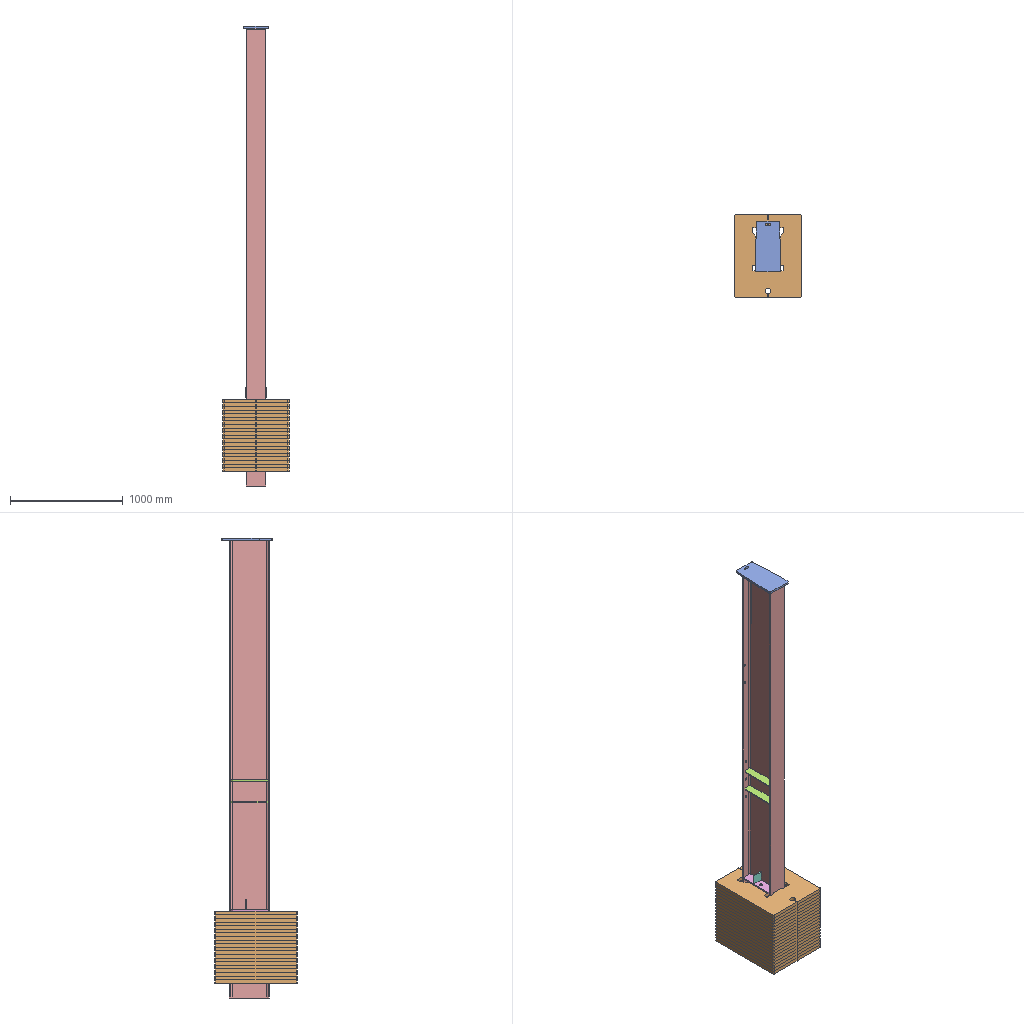Assembly | SolidWorks | 6 different items | 30 placed | box 592 x 737 x 4083 mm
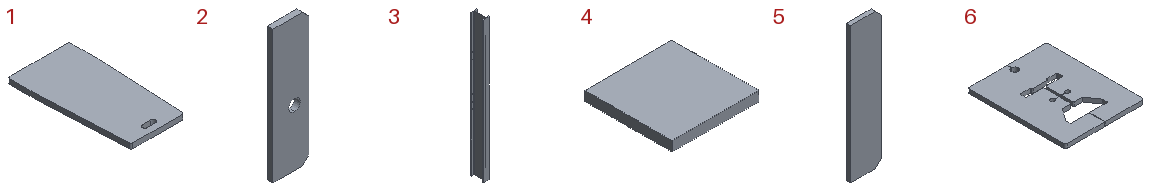Parts list (item | quantity | size | volume | features):
1 | x1 | 230 x 447.55 x 19.05 mm | 1843027 mm3 | features Extrusion 1
2 | x2 | 88.9 x 14 x 330.2 mm | 398595 mm3 | features Extrusion 1
3 | x1 | 171.323 x 355.092 x 4064 mm | 26304101 mm3 | features Chamfer 1, Extrusion 1, ICE 1, SketchHole 1
4 | x2 | 88.9 x 88.9 x 10 mm | 79032 mm3 | features Extrusion 1
5 | x4 | 76.2 x 10 x 330.2 mm | 249132 mm3 | features Extrusion 1
6 | x20 | 591.82 x 736.6 x 32 mm | 12345944 mm3 | features Extrusion 1
Mates (type | each side: item.copy, entity, surface, feature):
Coincident | 3.1 plane | assembly plane | 2 times
Coincident | 3.1 select_type:25 | assembly plane
Coincident | 1.1 plane | assembly plane
Coincident | 3.1 face plane Boss-Extrude1 | 1.1 face plane Boss-Extrude1
DistanceDim | 3.1 face plane Boss-Extrude1 | 1.1 face plane Boss-Extrude1
Coincident | 3.1 face plane Boss-Extrude1 | 5.1 face plane Boss-Extrude1 | 2 times
DistanceDim | 5.1 face plane Boss-Extrude1 | 1.1 face plane Boss-Extrude1
Coincident | 3.1 face plane Boss-Extrude1 | 2.1 face plane Boss-Extrude1
Coincident | 2.1 face plane Boss-Extrude1 | 3.1 face plane Boss-Extrude1
DistanceDim | 2.1 face plane Boss-Extrude1 | 3.1 face plane Boss-Extrude1
Coincident | 2.1 face plane Boss-Extrude1 | 4.1 face plane Boss-Extrude1
Coincident | 3.1 face plane Boss-Extrude1 | 4.1 face plane Boss-Extrude1
DistanceDim | 4.1 face plane Boss-Extrude1 | 3.1 face plane Boss-Extrude1
Symmetric | 6.1 face plane Boss-Extrude1 | 6.1 face plane Boss-Extrude1 | assembly plane
Coincident | 3.1 face plane Boss-Extrude1 | 6.1 face plane Boss-Extrude1
Coincident | 2.1 face plane Boss-Extrude1 | 6.1 face plane Boss-Extrude1